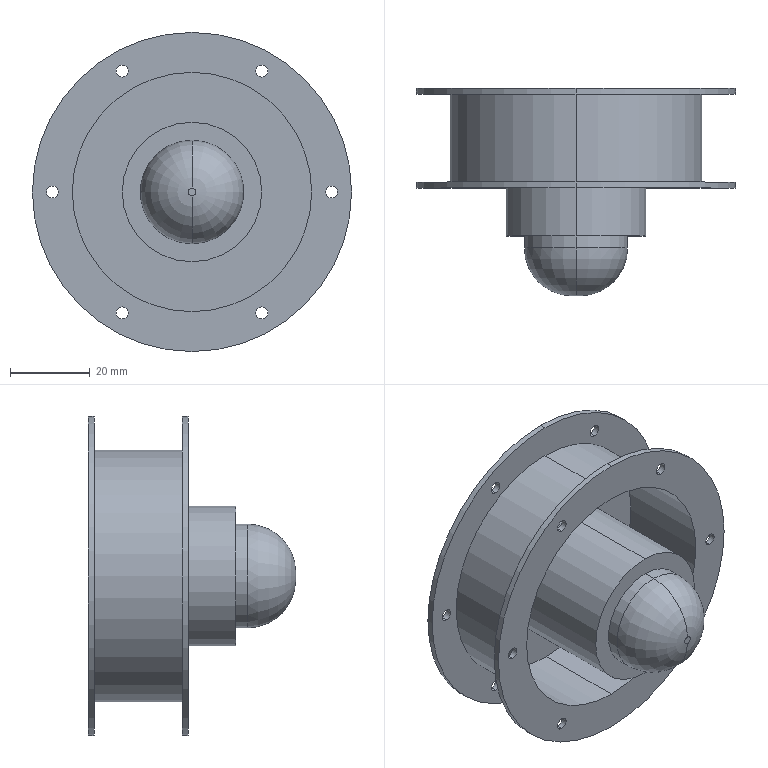Part | SolidWorks | features ICE 5, Fillet 1, Revolution 1 | 1 solid | 48 faces | box 80 x 52 x 80 mm | volume 58059 mm3 | cylinder 38 | plane 8 | torus 2 | commonest cylinder face diameters 3 x24 80 x4 6.964 x2 26 x2 35 x2 60 x2
STEP:
#1=CARTESIAN_POINT('',(0.,-15.,13.));
#2=VERTEX_POINT('',#1);
#3=CARTESIAN_POINT('',(0.,-15.,-13.));
#4=VERTEX_POINT('',#3);
#5=CARTESIAN_POINT('',(0.,-15.,0.));
#6=DIRECTION('',(0.,1.,0.));
#7=DIRECTION('',(0.,0.,-1.));
#8=AXIS2_PLACEMENT_3D('',#5,#6,#7);
#9=CIRCLE('',#8,13.);
#10=EDGE_CURVE('',#2,#4,#9,.T.);
#11=ORIENTED_EDGE('',*,*,#10,.F.);
#12=CARTESIAN_POINT('',(0.,-27.,1.));
#13=VERTEX_POINT('',#12);
#14=CARTESIAN_POINT('',(0.,-15.,1.));
#15=DIRECTION('',(1.,0.,0.));
#16=DIRECTION('',(0.,0.,-1.));
#17=AXIS2_PLACEMENT_3D('',#14,#15,#16);
#18=CIRCLE('',#17,12.);
#19=EDGE_CURVE('',#2,#13,#18,.T.);
#20=ORIENTED_EDGE('',*,*,#19,.T.);
#21=CARTESIAN_POINT('',(0.,-27.,-1.));
#22=VERTEX_POINT('',#21);
#23=CARTESIAN_POINT('',(0.,-27.,0.));
#24=DIRECTION('',(0.,-1.,0.));
#25=DIRECTION('',(0.,0.,-1.));
#26=AXIS2_PLACEMENT_3D('',#23,#24,#25);
#27=CIRCLE('',#26,1.);
#28=EDGE_CURVE('',#22,#13,#27,.T.);
#29=ORIENTED_EDGE('',*,*,#28,.F.);
#30=CARTESIAN_POINT('',(0.,-15.,-1.));
#31=DIRECTION('',(-1.,0.,0.));
#32=DIRECTION('',(0.,0.,1.));
#33=AXIS2_PLACEMENT_3D('',#30,#31,#32);
#34=CIRCLE('',#33,12.);
#35=EDGE_CURVE('',#4,#22,#34,.T.);
#36=ORIENTED_EDGE('',*,*,#35,.F.);
#37=EDGE_LOOP('',(#11,#20,#29,#36));
#38=FACE_OUTER_BOUND('',#37,.T.);
#39=CARTESIAN_POINT('',(0.,-15.,0.));
#40=DIRECTION('',(0.,-1.,0.));
#41=DIRECTION('',(0.,0.,-1.));
#42=AXIS2_PLACEMENT_3D('',#39,#40,#41);
#43=TOROIDAL_SURFACE('',#42,1.,12.);
#44=ADVANCED_FACE('',(#38),#43,.T.);
#45=ORIENTED_EDGE('',*,*,#10,.T.);
#46=CARTESIAN_POINT('',(0.,-12.,-13.));
#47=VERTEX_POINT('',#46);
#48=CARTESIAN_POINT('',(0.,-27.,-13.));
#49=DIRECTION('',(0.,1.,0.));
#50=VECTOR('',#49,1000.);
#51=LINE('',#48,#50);
#52=EDGE_CURVE('',#4,#47,#51,.T.);
#53=ORIENTED_EDGE('',*,*,#52,.T.);
#54=CARTESIAN_POINT('',(0.,-12.,13.));
#55=VERTEX_POINT('',#54);
#56=CARTESIAN_POINT('',(0.,-12.,0.));
#57=DIRECTION('',(0.,-1.,0.));
#58=DIRECTION('',(0.,0.,-1.));
#59=AXIS2_PLACEMENT_3D('',#56,#57,#58);
#60=CIRCLE('',#59,13.);
#61=EDGE_CURVE('',#47,#55,#60,.T.);
#62=ORIENTED_EDGE('',*,*,#61,.T.);
#63=CARTESIAN_POINT('',(0.,-27.,13.));
#64=DIRECTION('',(0.,1.,0.));
#65=VECTOR('',#64,1000.);
#66=LINE('',#63,#65);
#67=EDGE_CURVE('',#2,#55,#66,.T.);
#68=ORIENTED_EDGE('',*,*,#67,.F.);
#69=EDGE_LOOP('',(#45,#53,#62,#68));
#70=FACE_OUTER_BOUND('',#69,.T.);
#71=CARTESIAN_POINT('',(0.,-27.,0.));
#72=DIRECTION('',(0.,1.,0.));
#73=DIRECTION('',(0.,0.,1.));
#74=AXIS2_PLACEMENT_3D('',#71,#72,#73);
#75=CYLINDRICAL_SURFACE('',#74,13.);
#76=ADVANCED_FACE('',(#70),#75,.T.);
#77=CARTESIAN_POINT('',(0.,-12.,-17.5));
#78=VERTEX_POINT('',#77);
#79=CARTESIAN_POINT('',(0.,-12.,17.5));
#80=VERTEX_POINT('',#79);
#81=CARTESIAN_POINT('',(0.,-12.,0.));
#82=DIRECTION('',(0.,-1.,0.));
#83=DIRECTION('',(0.,0.,-1.));
#84=AXIS2_PLACEMENT_3D('',#81,#82,#83);
#85=CIRCLE('',#84,17.5);
#86=EDGE_CURVE('',#78,#80,#85,.T.);
#87=ORIENTED_EDGE('',*,*,#86,.F.);
#88=CARTESIAN_POINT('',(0.,23.,-17.5));
#89=VERTEX_POINT('',#88);
#90=CARTESIAN_POINT('',(0.,-12.,-17.5));
#91=DIRECTION('',(0.,1.,0.));
#92=VECTOR('',#91,1000.);
#93=LINE('',#90,#92);
#94=EDGE_CURVE('',#78,#89,#93,.T.);
#95=ORIENTED_EDGE('',*,*,#94,.T.);
#96=CARTESIAN_POINT('',(0.,23.,17.5));
#97=VERTEX_POINT('',#96);
#98=CARTESIAN_POINT('',(0.,23.,0.));
#99=DIRECTION('',(0.,-1.,0.));
#100=DIRECTION('',(0.,0.,1.));
#101=AXIS2_PLACEMENT_3D('',#98,#99,#100);
#102=CIRCLE('',#101,17.5);
#103=EDGE_CURVE('',#89,#97,#102,.T.);
#104=ORIENTED_EDGE('',*,*,#103,.T.);
#105=CARTESIAN_POINT('',(0.,-12.,17.5));
#106=DIRECTION('',(0.,1.,0.));
#107=VECTOR('',#106,1000.);
#108=LINE('',#105,#107);
#109=EDGE_CURVE('',#80,#97,#108,.T.);
#110=ORIENTED_EDGE('',*,*,#109,.F.);
#111=EDGE_LOOP('',(#87,#95,#104,#110));
#112=FACE_OUTER_BOUND('',#111,.T.);
#113=CARTESIAN_POINT('',(0.,-12.,0.));
#114=DIRECTION('',(0.,1.,0.));
#115=DIRECTION('',(0.,0.,1.));
#116=AXIS2_PLACEMENT_3D('',#113,#114,#115);
#117=CYLINDRICAL_SURFACE('',#116,17.5);
#118=ADVANCED_FACE('',(#112),#117,.T.);
#119=CARTESIAN_POINT('',(0.,25.,3.482));
#120=VERTEX_POINT('',#119);
#121=CARTESIAN_POINT('',(0.,25.,-3.482));
#122=VERTEX_POINT('',#121);
#123=CARTESIAN_POINT('',(0.,25.,0.));
#124=DIRECTION('',(0.,-1.,0.));
#125=DIRECTION('',(0.,0.,-1.));
#126=AXIS2_PLACEMENT_3D('',#123,#124,#125);
#127=CIRCLE('',#126,3.482);
#128=EDGE_CURVE('',#120,#122,#127,.T.);
#129=ORIENTED_EDGE('',*,*,#128,.F.);
#130=CARTESIAN_POINT('',(0.,23.,3.482));
#131=VERTEX_POINT('',#130);
#132=CARTESIAN_POINT('',(0.,25.,3.482));
#133=DIRECTION('',(0.,-1.,0.));
#134=VECTOR('',#133,1000.);
#135=LINE('',#132,#134);
#136=EDGE_CURVE('',#120,#131,#135,.T.);
#137=ORIENTED_EDGE('',*,*,#136,.T.);
#138=CARTESIAN_POINT('',(0.,23.,-3.482));
#139=VERTEX_POINT('',#138);
#140=CARTESIAN_POINT('',(0.,23.,0.));
#141=DIRECTION('',(0.,1.,0.));
#142=DIRECTION('',(0.,0.,-1.));
#143=AXIS2_PLACEMENT_3D('',#140,#141,#142);
#144=CIRCLE('',#143,3.482);
#145=EDGE_CURVE('',#139,#131,#144,.T.);
#146=ORIENTED_EDGE('',*,*,#145,.F.);
#147=CARTESIAN_POINT('',(0.,25.,-3.482));
#148=DIRECTION('',(0.,-1.,0.));
#149=VECTOR('',#148,1000.);
#150=LINE('',#147,#149);
#151=EDGE_CURVE('',#122,#139,#150,.T.);
#152=ORIENTED_EDGE('',*,*,#151,.F.);
#153=EDGE_LOOP('',(#129,#137,#146,#152));
#154=FACE_OUTER_BOUND('',#153,.T.);
#155=CARTESIAN_POINT('',(0.,25.,0.));
#156=DIRECTION('',(0.,-1.,0.));
#157=DIRECTION('',(0.,0.,-1.));
#158=AXIS2_PLACEMENT_3D('',#155,#156,#157);
#159=CYLINDRICAL_SURFACE('',#158,3.482);
#160=ADVANCED_FACE('',(#154),#159,.F.);
#161=CARTESIAN_POINT('',(-17.5,23.5,-31.811));
#162=VERTEX_POINT('',#161);
#163=CARTESIAN_POINT('',(-17.5,23.5,-28.811));
#164=VERTEX_POINT('',#163);
#165=CARTESIAN_POINT('',(-17.5,23.5,-30.311));
#166=DIRECTION('',(0.,1.,0.));
#167=DIRECTION('',(0.,0.,1.));
#168=AXIS2_PLACEMENT_3D('',#165,#166,#167);
#169=CIRCLE('',#168,1.5);
#170=EDGE_CURVE('',#162,#164,#169,.T.);
#171=ORIENTED_EDGE('',*,*,#170,.F.);
#172=CARTESIAN_POINT('',(-17.5,25.,-31.811));
#173=VERTEX_POINT('',#172);
#174=CARTESIAN_POINT('',(-17.5,0.,-31.811));
#175=DIRECTION('',(0.,1.,0.));
#176=VECTOR('',#175,1000.);
#177=LINE('',#174,#176);
#178=EDGE_CURVE('',#162,#173,#177,.T.);
#179=ORIENTED_EDGE('',*,*,#178,.T.);
#180=CARTESIAN_POINT('',(-17.5,25.,-28.811));
#181=VERTEX_POINT('',#180);
#182=CARTESIAN_POINT('',(-17.5,25.,-30.311));
#183=DIRECTION('',(0.,1.,0.));
#184=DIRECTION('',(0.,0.,1.));
#185=AXIS2_PLACEMENT_3D('',#182,#183,#184);
#186=CIRCLE('',#185,1.5);
#187=EDGE_CURVE('',#173,#181,#186,.T.);
#188=ORIENTED_EDGE('',*,*,#187,.T.);
#189=CARTESIAN_POINT('',(-17.5,0.,-28.811));
#190=DIRECTION('',(0.,1.,0.));
#191=VECTOR('',#190,1000.);
#192=LINE('',#189,#191);
#193=EDGE_CURVE('',#164,#181,#192,.T.);
#194=ORIENTED_EDGE('',*,*,#193,.F.);
#195=EDGE_LOOP('',(#171,#179,#188,#194));
#196=FACE_OUTER_BOUND('',#195,.T.);
#197=CARTESIAN_POINT('',(-17.5,0.,-30.311));
#198=DIRECTION('',(0.,1.,0.));
#199=DIRECTION('',(0.,0.,1.));
#200=AXIS2_PLACEMENT_3D('',#197,#198,#199);
#201=CYLINDRICAL_SURFACE('',#200,1.5);
#202=ADVANCED_FACE('',(#196),#201,.F.);
#203=CARTESIAN_POINT('',(17.5,23.5,-31.811));
#204=VERTEX_POINT('',#203);
#205=CARTESIAN_POINT('',(17.5,23.5,-28.811));
#206=VERTEX_POINT('',#205);
#207=CARTESIAN_POINT('',(17.5,23.5,-30.311));
#208=DIRECTION('',(0.,1.,0.));
#209=DIRECTION('',(0.,0.,1.));
#210=AXIS2_PLACEMENT_3D('',#207,#208,#209);
#211=CIRCLE('',#210,1.5);
#212=EDGE_CURVE('',#204,#206,#211,.T.);
#213=ORIENTED_EDGE('',*,*,#212,.F.);
#214=CARTESIAN_POINT('',(17.5,25.,-31.811));
#215=VERTEX_POINT('',#214);
#216=CARTESIAN_POINT('',(17.5,0.,-31.811));
#217=DIRECTION('',(0.,1.,0.));
#218=VECTOR('',#217,1000.);
#219=LINE('',#216,#218);
#220=EDGE_CURVE('',#204,#215,#219,.T.);
#221=ORIENTED_EDGE('',*,*,#220,.T.);
#222=CARTESIAN_POINT('',(17.5,25.,-28.811));
#223=VERTEX_POINT('',#222);
#224=CARTESIAN_POINT('',(17.5,25.,-30.311));
#225=DIRECTION('',(0.,1.,0.));
#226=DIRECTION('',(0.,0.,1.));
#227=AXIS2_PLACEMENT_3D('',#224,#225,#226);
#228=CIRCLE('',#227,1.5);
#229=EDGE_CURVE('',#215,#223,#228,.T.);
#230=ORIENTED_EDGE('',*,*,#229,.T.);
#231=CARTESIAN_POINT('',(17.5,0.,-28.811));
#232=DIRECTION('',(0.,1.,0.));
#233=VECTOR('',#232,1000.);
#234=LINE('',#231,#233);
#235=EDGE_CURVE('',#206,#223,#234,.T.);
#236=ORIENTED_EDGE('',*,*,#235,.F.);
#237=EDGE_LOOP('',(#213,#221,#230,#236));
#238=FACE_OUTER_BOUND('',#237,.T.);
#239=CARTESIAN_POINT('',(17.5,0.,-30.311));
#240=DIRECTION('',(0.,1.,0.));
#241=DIRECTION('',(0.,0.,1.));
#242=AXIS2_PLACEMENT_3D('',#239,#240,#241);
#243=CYLINDRICAL_SURFACE('',#242,1.5);
#244=ADVANCED_FACE('',(#238),#243,.F.);
#245=CARTESIAN_POINT('',(35.,23.5,-1.5));
#246=VERTEX_POINT('',#245);
#247=CARTESIAN_POINT('',(35.,23.5,1.5));
#248=VERTEX_POINT('',#247);
#249=CARTESIAN_POINT('',(35.,23.5,0.));
#250=DIRECTION('',(0.,1.,0.));
#251=DIRECTION('',(0.,0.,1.));
#252=AXIS2_PLACEMENT_3D('',#249,#250,#251);
#253=CIRCLE('',#252,1.5);
#254=EDGE_CURVE('',#246,#248,#253,.T.);
#255=ORIENTED_EDGE('',*,*,#254,.F.);
#256=CARTESIAN_POINT('',(35.,25.,-1.5));
#257=VERTEX_POINT('',#256);
#258=CARTESIAN_POINT('',(35.,0.,-1.5));
#259=DIRECTION('',(0.,1.,0.));
#260=VECTOR('',#259,1000.);
#261=LINE('',#258,#260);
#262=EDGE_CURVE('',#246,#257,#261,.T.);
#263=ORIENTED_EDGE('',*,*,#262,.T.);
#264=CARTESIAN_POINT('',(35.,25.,1.5));
#265=VERTEX_POINT('',#264);
#266=CARTESIAN_POINT('',(35.,25.,0.));
#267=DIRECTION('',(0.,1.,0.));
#268=DIRECTION('',(0.,0.,1.));
#269=AXIS2_PLACEMENT_3D('',#266,#267,#268);
#270=CIRCLE('',#269,1.5);
#271=EDGE_CURVE('',#257,#265,#270,.T.);
#272=ORIENTED_EDGE('',*,*,#271,.T.);
#273=CARTESIAN_POINT('',(35.,0.,1.5));
#274=DIRECTION('',(0.,1.,0.));
#275=VECTOR('',#274,1000.);
#276=LINE('',#273,#275);
#277=EDGE_CURVE('',#248,#265,#276,.T.);
#278=ORIENTED_EDGE('',*,*,#277,.F.);
#279=EDGE_LOOP('',(#255,#263,#272,#278));
#280=FACE_OUTER_BOUND('',#279,.T.);
#281=CARTESIAN_POINT('',(35.,0.,0.));
#282=DIRECTION('',(0.,1.,0.));
#283=DIRECTION('',(0.,0.,1.));
#284=AXIS2_PLACEMENT_3D('',#281,#282,#283);
#285=CYLINDRICAL_SURFACE('',#284,1.5);
#286=ADVANCED_FACE('',(#280),#285,.F.);
#287=CARTESIAN_POINT('',(17.5,23.5,28.811));
#288=VERTEX_POINT('',#287);
#289=CARTESIAN_POINT('',(17.5,23.5,31.811));
#290=VERTEX_POINT('',#289);
#291=CARTESIAN_POINT('',(17.5,23.5,30.311));
#292=DIRECTION('',(0.,1.,0.));
#293=DIRECTION('',(0.,0.,1.));
#294=AXIS2_PLACEMENT_3D('',#291,#292,#293);
#295=CIRCLE('',#294,1.5);
#296=EDGE_CURVE('',#288,#290,#295,.T.);
#297=ORIENTED_EDGE('',*,*,#296,.F.);
#298=CARTESIAN_POINT('',(17.5,25.,28.811));
#299=VERTEX_POINT('',#298);
#300=CARTESIAN_POINT('',(17.5,0.,28.811));
#301=DIRECTION('',(0.,1.,0.));
#302=VECTOR('',#301,1000.);
#303=LINE('',#300,#302);
#304=EDGE_CURVE('',#288,#299,#303,.T.);
#305=ORIENTED_EDGE('',*,*,#304,.T.);
#306=CARTESIAN_POINT('',(17.5,25.,31.811));
#307=VERTEX_POINT('',#306);
#308=CARTESIAN_POINT('',(17.5,25.,30.311));
#309=DIRECTION('',(0.,1.,0.));
#310=DIRECTION('',(0.,0.,1.));
#311=AXIS2_PLACEMENT_3D('',#308,#309,#310);
#312=CIRCLE('',#311,1.5);
#313=EDGE_CURVE('',#299,#307,#312,.T.);
#314=ORIENTED_EDGE('',*,*,#313,.T.);
#315=CARTESIAN_POINT('',(17.5,0.,31.811));
#316=DIRECTION('',(0.,1.,0.));
#317=VECTOR('',#316,1000.);
#318=LINE('',#315,#317);
#319=EDGE_CURVE('',#290,#307,#318,.T.);
#320=ORIENTED_EDGE('',*,*,#319,.F.);
#321=EDGE_LOOP('',(#297,#305,#314,#320));
#322=FACE_OUTER_BOUND('',#321,.T.);
#323=CARTESIAN_POINT('',(17.5,0.,30.311));
#324=DIRECTION('',(0.,1.,0.));
#325=DIRECTION('',(0.,0.,1.));
#326=AXIS2_PLACEMENT_3D('',#323,#324,#325);
#327=CYLINDRICAL_SURFACE('',#326,1.5);
#328=ADVANCED_FACE('',(#322),#327,.F.);
#329=CARTESIAN_POINT('',(-17.5,23.5,28.811));
#330=VERTEX_POINT('',#329);
#331=CARTESIAN_POINT('',(-17.5,23.5,31.811));
#332=VERTEX_POINT('',#331);
#333=CARTESIAN_POINT('',(-17.5,23.5,30.311));
#334=DIRECTION('',(0.,1.,0.));
#335=DIRECTION('',(0.,0.,1.));
#336=AXIS2_PLACEMENT_3D('',#333,#334,#335);
#337=CIRCLE('',#336,1.5);
#338=EDGE_CURVE('',#330,#332,#337,.T.);
#339=ORIENTED_EDGE('',*,*,#338,.F.);
#340=CARTESIAN_POINT('',(-17.5,25.,28.811));
#341=VERTEX_POINT('',#340);
#342=CARTESIAN_POINT('',(-17.5,0.,28.811));
#343=DIRECTION('',(0.,1.,0.));
#344=VECTOR('',#343,1000.);
#345=LINE('',#342,#344);
#346=EDGE_CURVE('',#330,#341,#345,.T.);
#347=ORIENTED_EDGE('',*,*,#346,.T.);
#348=CARTESIAN_POINT('',(-17.5,25.,31.811));
#349=VERTEX_POINT('',#348);
#350=CARTESIAN_POINT('',(-17.5,25.,30.311));
#351=DIRECTION('',(0.,1.,0.));
#352=DIRECTION('',(0.,0.,1.));
#353=AXIS2_PLACEMENT_3D('',#350,#351,#352);
#354=CIRCLE('',#353,1.5);
#355=EDGE_CURVE('',#341,#349,#354,.T.);
#356=ORIENTED_EDGE('',*,*,#355,.T.);
#357=CARTESIAN_POINT('',(-17.5,0.,31.811));
#358=DIRECTION('',(0.,1.,0.));
#359=VECTOR('',#358,1000.);
#360=LINE('',#357,#359);
#361=EDGE_CURVE('',#332,#349,#360,.T.);
#362=ORIENTED_EDGE('',*,*,#361,.F.);
#363=EDGE_LOOP('',(#339,#347,#356,#362));
#364=FACE_OUTER_BOUND('',#363,.T.);
#365=CARTESIAN_POINT('',(-17.5,0.,30.311));
#366=DIRECTION('',(0.,1.,0.));
#367=DIRECTION('',(0.,0.,1.));
#368=AXIS2_PLACEMENT_3D('',#365,#366,#367);
#369=CYLINDRICAL_SURFACE('',#368,1.5);
#370=ADVANCED_FACE('',(#364),#369,.F.);
#371=CARTESIAN_POINT('',(-17.5,0.,-31.811));
#372=VERTEX_POINT('',#371);
#373=CARTESIAN_POINT('',(-17.5,0.,-28.811));
#374=VERTEX_POINT('',#373);
#375=CARTESIAN_POINT('',(-17.5,0.,-30.311));
#376=DIRECTION('',(0.,1.,0.));
#377=DIRECTION('',(0.,0.,1.));
#378=AXIS2_PLACEMENT_3D('',#375,#376,#377);
#379=CIRCLE('',#378,1.5);
#380=EDGE_CURVE('',#372,#374,#379,.T.);
#381=ORIENTED_EDGE('',*,*,#380,.F.);
#382=CARTESIAN_POINT('',(-17.5,1.5,-31.811));
#383=VERTEX_POINT('',#382);
#384=CARTESIAN_POINT('',(-17.5,0.,-31.811));
#385=DIRECTION('',(0.,1.,0.));
#386=VECTOR('',#385,1000.);
#387=LINE('',#384,#386);
#388=EDGE_CURVE('',#372,#383,#387,.T.);
#389=ORIENTED_EDGE('',*,*,#388,.T.);
#390=CARTESIAN_POINT('',(-17.5,1.5,-28.811));
#391=VERTEX_POINT('',#390);
#392=CARTESIAN_POINT('',(-17.5,1.5,-30.311));
#393=DIRECTION('',(0.,-1.,0.));
#394=DIRECTION('',(0.,0.,-1.));
#395=AXIS2_PLACEMENT_3D('',#392,#393,#394);
#396=CIRCLE('',#395,1.5);
#397=EDGE_CURVE('',#391,#383,#396,.T.);
#398=ORIENTED_EDGE('',*,*,#397,.F.);
#399=CARTESIAN_POINT('',(-17.5,0.,-28.811));
#400=DIRECTION('',(0.,1.,0.));
#401=VECTOR('',#400,1000.);
#402=LINE('',#399,#401);
#403=EDGE_CURVE('',#374,#391,#402,.T.);
#404=ORIENTED_EDGE('',*,*,#403,.F.);
#405=EDGE_LOOP('',(#381,#389,#398,#404));
#406=FACE_OUTER_BOUND('',#405,.T.);
#407=CARTESIAN_POINT('',(-17.5,0.,-30.311));
#408=DIRECTION('',(0.,1.,0.));
#409=DIRECTION('',(0.,0.,1.));
#410=AXIS2_PLACEMENT_3D('',#407,#408,#409);
#411=CYLINDRICAL_SURFACE('',#410,1.5);
#412=ADVANCED_FACE('',(#406),#411,.F.);
#413=CARTESIAN_POINT('',(17.5,0.,-31.811));
#414=VERTEX_POINT('',#413);
#415=CARTESIAN_POINT('',(17.5,0.,-28.811));
#416=VERTEX_POINT('',#415);
#417=CARTESIAN_POINT('',(17.5,0.,-30.311));
#418=DIRECTION('',(0.,1.,0.));
#419=DIRECTION('',(0.,0.,1.));
#420=AXIS2_PLACEMENT_3D('',#417,#418,#419);
#421=CIRCLE('',#420,1.5);
#422=EDGE_CURVE('',#414,#416,#421,.T.);
#423=ORIENTED_EDGE('',*,*,#422,.F.);
#424=CARTESIAN_POINT('',(17.5,1.5,-31.811));
#425=VERTEX_POINT('',#424);
#426=CARTESIAN_POINT('',(17.5,0.,-31.811));
#427=DIRECTION('',(0.,1.,0.));
#428=VECTOR('',#427,1000.);
#429=LINE('',#426,#428);
#430=EDGE_CURVE('',#414,#425,#429,.T.);
#431=ORIENTED_EDGE('',*,*,#430,.T.);
#432=CARTESIAN_POINT('',(17.5,1.5,-28.811));
#433=VERTEX_POINT('',#432);
#434=CARTESIAN_POINT('',(17.5,1.5,-30.311));
#435=DIRECTION('',(0.,-1.,0.));
#436=DIRECTION('',(0.,0.,-1.));
#437=AXIS2_PLACEMENT_3D('',#434,#435,#436);
#438=CIRCLE('',#437,1.5);
#439=EDGE_CURVE('',#433,#425,#438,.T.);
#440=ORIENTED_EDGE('',*,*,#439,.F.);
#441=CARTESIAN_POINT('',(17.5,0.,-28.811));
#442=DIRECTION('',(0.,1.,0.));
#443=VECTOR('',#442,1000.);
#444=LINE('',#441,#443);
#445=EDGE_CURVE('',#416,#433,#444,.T.);
#446=ORIENTED_EDGE('',*,*,#445,.F.);
#447=EDGE_LOOP('',(#423,#431,#440,#446));
#448=FACE_OUTER_BOUND('',#447,.T.);
#449=CARTESIAN_POINT('',(17.5,0.,-30.311));
#450=DIRECTION('',(0.,1.,0.));
#451=DIRECTION('',(0.,0.,1.));
#452=AXIS2_PLACEMENT_3D('',#449,#450,#451);
#453=CYLINDRICAL_SURFACE('',#452,1.5);
#454=ADVANCED_FACE('',(#448),#453,.F.);
#455=CARTESIAN_POINT('',(35.,0.,-1.5));
#456=VERTEX_POINT('',#455);
#457=CARTESIAN_POINT('',(35.,0.,1.5));
#458=VERTEX_POINT('',#457);
#459=CARTESIAN_POINT('',(35.,0.,0.));
#460=DIRECTION('',(0.,1.,0.));
#461=DIRECTION('',(0.,0.,1.));
#462=AXIS2_PLACEMENT_3D('',#459,#460,#461);
#463=CIRCLE('',#462,1.5);
#464=EDGE_CURVE('',#456,#458,#463,.T.);
#465=ORIENTED_EDGE('',*,*,#464,.F.);
#466=CARTESIAN_POINT('',(35.,1.5,-1.5));
#467=VERTEX_POINT('',#466);
#468=CARTESIAN_POINT('',(35.,0.,-1.5));
#469=DIRECTION('',(0.,1.,0.));
#470=VECTOR('',#469,1000.);
#471=LINE('',#468,#470);
#472=EDGE_CURVE('',#456,#467,#471,.T.);
#473=ORIENTED_EDGE('',*,*,#472,.T.);
#474=CARTESIAN_POINT('',(35.,1.5,1.5));
#475=VERTEX_POINT('',#474);
#476=CARTESIAN_POINT('',(35.,1.5,0.));
#477=DIRECTION('',(0.,-1.,0.));
#478=DIRECTION('',(0.,0.,-1.));
#479=AXIS2_PLACEMENT_3D('',#476,#477,#478);
#480=CIRCLE('',#479,1.5);
#481=EDGE_CURVE('',#475,#467,#480,.T.);
#482=ORIENTED_EDGE('',*,*,#481,.F.);
#483=CARTESIAN_POINT('',(35.,0.,1.5));
#484=DIRECTION('',(0.,1.,0.));
#485=VECTOR('',#484,1000.);
#486=LINE('',#483,#485);
#487=EDGE_CURVE('',#458,#475,#486,.T.);
#488=ORIENTED_EDGE('',*,*,#487,.F.);
#489=EDGE_LOOP('',(#465,#473,#482,#488));
#490=FACE_OUTER_BOUND('',#489,.T.);
#491=CARTESIAN_POINT('',(35.,0.,0.));
#492=DIRECTION('',(0.,1.,0.));
#493=DIRECTION('',(0.,0.,1.));
#494=AXIS2_PLACEMENT_3D('',#491,#492,#493);
#495=CYLINDRICAL_SURFACE('',#494,1.5);
#496=ADVANCED_FACE('',(#490),#495,.F.);
#497=CARTESIAN_POINT('',(17.5,0.,28.811));
#498=VERTEX_POINT('',#497);
#499=CARTESIAN_POINT('',(17.5,0.,31.811));
#500=VERTEX_POINT('',#499);
#501=CARTESIAN_POINT('',(17.5,0.,30.311));
#502=DIRECTION('',(0.,1.,0.));
#503=DIRECTION('',(0.,0.,1.));
#504=AXIS2_PLACEMENT_3D('',#501,#502,#503);
#505=CIRCLE('',#504,1.5);
#506=EDGE_CURVE('',#498,#500,#505,.T.);
#507=ORIENTED_EDGE('',*,*,#506,.F.);
#508=CARTESIAN_POINT('',(17.5,1.5,28.811));
#509=VERTEX_POINT('',#508);
#510=CARTESIAN_POINT('',(17.5,0.,28.811));
#511=DIRECTION('',(0.,1.,0.));
#512=VECTOR('',#511,1000.);
#513=LINE('',#510,#512);
#514=EDGE_CURVE('',#498,#509,#513,.T.);
#515=ORIENTED_EDGE('',*,*,#514,.T.);
#516=CARTESIAN_POINT('',(17.5,1.5,31.811));
#517=VERTEX_POINT('',#516);
#518=CARTESIAN_POINT('',(17.5,1.5,30.311));
#519=DIRECTION('',(0.,-1.,0.));
#520=DIRECTION('',(0.,0.,-1.));
#521=AXIS2_PLACEMENT_3D('',#518,#519,#520);
#522=CIRCLE('',#521,1.5);
#523=EDGE_CURVE('',#517,#509,#522,.T.);
#524=ORIENTED_EDGE('',*,*,#523,.F.);
#525=CARTESIAN_POINT('',(17.5,0.,31.811));
#526=DIRECTION('',(0.,1.,0.));
#527=VECTOR('',#526,1000.);
#528=LINE('',#525,#527);
#529=EDGE_CURVE('',#500,#517,#528,.T.);
#530=ORIENTED_EDGE('',*,*,#529,.F.);
#531=EDGE_LOOP('',(#507,#515,#524,#530));
#532=FACE_OUTER_BOUND('',#531,.T.);
#533=CARTESIAN_POINT('',(17.5,0.,30.311));
#534=DIRECTION('',(0.,1.,0.));
#535=DIRECTION('',(0.,0.,1.));
#536=AXIS2_PLACEMENT_3D('',#533,#534,#535);
#537=CYLINDRICAL_SURFACE('',#536,1.5);
#538=ADVANCED_FACE('',(#532),#537,.F.);
#539=CARTESIAN_POINT('',(-17.5,0.,28.811));
#540=VERTEX_POINT('',#539);
#541=CARTESIAN_POINT('',(-17.5,0.,31.811));
#542=VERTEX_POINT('',#541);
#543=CARTESIAN_POINT('',(-17.5,0.,30.311));
#544=DIRECTION('',(0.,1.,0.));
#545=DIRECTION('',(0.,0.,1.));
#546=AXIS2_PLACEMENT_3D('',#543,#544,#545);
#547=CIRCLE('',#546,1.5);
#548=EDGE_CURVE('',#540,#542,#547,.T.);
#549=ORIENTED_EDGE('',*,*,#548,.F.);
#550=CARTESIAN_POINT('',(-17.5,1.5,28.811));
#551=VERTEX_POINT('',#550);
#552=CARTESIAN_POINT('',(-17.5,0.,28.811));
#553=DIRECTION('',(0.,1.,0.));
#554=VECTOR('',#553,1000.);
#555=LINE('',#552,#554);
#556=EDGE_CURVE('',#540,#551,#555,.T.);
#557=ORIENTED_EDGE('',*,*,#556,.T.);
#558=CARTESIAN_POINT('',(-17.5,1.5,31.811));
#559=VERTEX_POINT('',#558);
#560=CARTESIAN_POINT('',(-17.5,1.5,30.311));
#561=DIRECTION('',(0.,-1.,0.));
#562=DIRECTION('',(0.,0.,-1.));
#563=AXIS2_PLACEMENT_3D('',#560,#561,#562);
#564=CIRCLE('',#563,1.5);
#565=EDGE_CURVE('',#559,#551,#564,.T.);
#566=ORIENTED_EDGE('',*,*,#565,.F.);
#567=CARTESIAN_POINT('',(-17.5,0.,31.811));
#568=DIRECTION('',(0.,1.,0.));
#569=VECTOR('',#568,1000.);
#570=LINE('',#567,#569);
#571=EDGE_CURVE('',#542,#559,#570,.T.);
#572=ORIENTED_EDGE('',*,*,#571,.F.);
#573=EDGE_LOOP('',(#549,#557,#566,#572));
#574=FACE_OUTER_BOUND('',#573,.T.);
#575=CARTESIAN_POINT('',(-17.5,0.,30.311));
#576=DIRECTION('',(0.,1.,0.));
#577=DIRECTION('',(0.,0.,1.));
#578=AXIS2_PLACEMENT_3D('',#575,#576,#577);
#579=CYLINDRICAL_SURFACE('',#578,1.5);
#580=ADVANCED_FACE('',(#574),#579,.F.);
#581=CARTESIAN_POINT('',(-35.,23.5,-1.5));
#582=VERTEX_POINT('',#581);
#583=CARTESIAN_POINT('',(-35.,23.5,1.5));
#584=VERTEX_POINT('',#583);
#585=CARTESIAN_POINT('',(-35.,23.5,0.));
#586=DIRECTION('',(0.,1.,0.));
#587=DIRECTION('',(0.,0.,1.));
#588=AXIS2_PLACEMENT_3D('',#585,#586,#587);
#589=CIRCLE('',#588,1.5);
#590=EDGE_CURVE('',#582,#584,#589,.T.);
#591=ORIENTED_EDGE('',*,*,#590,.F.);
#592=CARTESIAN_POINT('',(-35.,25.,-1.5));
#593=VERTEX_POINT('',#592);
#594=CARTESIAN_POINT('',(-35.,0.,-1.5));
#595=DIRECTION('',(0.,1.,0.));
#596=VECTOR('',#595,1000.);
#597=LINE('',#594,#596);
#598=EDGE_CURVE('',#582,#593,#597,.T.);
#599=ORIENTED_EDGE('',*,*,#598,.T.);
#600=CARTESIAN_POINT('',(-35.,25.,1.5));
#601=VERTEX_POINT('',#600);
#602=CARTESIAN_POINT('',(-35.,25.,0.));
#603=DIRECTION('',(0.,1.,0.));
#604=DIRECTION('',(0.,0.,1.));
#605=AXIS2_PLACEMENT_3D('',#602,#603,#604);
#606=CIRCLE('',#605,1.5);
#607=EDGE_CURVE('',#593,#601,#606,.T.);
#608=ORIENTED_EDGE('',*,*,#607,.T.);
#609=CARTESIAN_POINT('',(-35.,0.,1.5));
#610=DIRECTION('',(0.,1.,0.));
#611=VECTOR('',#610,1000.);
#612=LINE('',#609,#611);
#613=EDGE_CURVE('',#584,#601,#612,.T.);
#614=ORIENTED_EDGE('',*,*,#613,.F.);
#615=EDGE_LOOP('',(#591,#599,#608,#614));
#616=FACE_OUTER_BOUND('',#615,.T.);
#617=CARTESIAN_POINT('',(-35.,0.,0.));
#618=DIRECTION('',(0.,1.,0.));
#619=DIRECTION('',(0.,0.,1.));
#620=AXIS2_PLACEMENT_3D('',#617,#618,#619);
#621=CYLINDRICAL_SURFACE('',#620,1.5);
#622=ADVANCED_FACE('',(#616),#621,.F.);
#623=CARTESIAN_POINT('',(-35.,0.,-1.5));
#624=VERTEX_POINT('',#623);
#625=CARTESIAN_POINT('',(-35.,0.,1.5));
#626=VERTEX_POINT('',#625);
#627=CARTESIAN_POINT('',(-35.,0.,0.));
#628=DIRECTION('',(0.,1.,0.));
#629=DIRECTION('',(0.,0.,1.));
#630=AXIS2_PLACEMENT_3D('',#627,#628,#629);
#631=CIRCLE('',#630,1.5);
#632=EDGE_CURVE('',#624,#626,#631,.T.);
#633=ORIENTED_EDGE('',*,*,#632,.F.);
#634=CARTESIAN_POINT('',(-35.,1.5,-1.5));
#635=VERTEX_POINT('',#634);
#636=CARTESIAN_POINT('',(-35.,0.,-1.5));
#637=DIRECTION('',(0.,1.,0.));
#638=VECTOR('',#637,1000.);
#639=LINE('',#636,#638);
#640=EDGE_CURVE('',#624,#635,#639,.T.);
#641=ORIENTED_EDGE('',*,*,#640,.T.);
#642=CARTESIAN_POINT('',(-35.,1.5,1.5));
#643=VERTEX_POINT('',#642);
#644=CARTESIAN_POINT('',(-35.,1.5,0.));
#645=DIRECTION('',(0.,-1.,0.));
#646=DIRECTION('',(0.,0.,-1.));
#647=AXIS2_PLACEMENT_3D('',#644,#645,#646);
#648=CIRCLE('',#647,1.5);
#649=EDGE_CURVE('',#643,#635,#648,.T.);
#650=ORIENTED_EDGE('',*,*,#649,.F.);
#651=CARTESIAN_POINT('',(-35.,0.,1.5));
#652=DIRECTION('',(0.,1.,0.));
#653=VECTOR('',#652,1000.);
#654=LINE('',#651,#653);
#655=EDGE_CURVE('',#626,#643,#654,.T.);
#656=ORIENTED_EDGE('',*,*,#655,.F.);
#657=EDGE_LOOP('',(#633,#641,#650,#656));
#658=FACE_OUTER_BOUND('',#657,.T.);
#659=CARTESIAN_POINT('',(-35.,0.,0.));
#660=DIRECTION('',(0.,1.,0.));
#661=DIRECTION('',(0.,0.,1.));
#662=AXIS2_PLACEMENT_3D('',#659,#660,#661);
#663=CYLINDRICAL_SURFACE('',#662,1.5);
#664=ADVANCED_FACE('',(#658),#663,.F.);
#665=CARTESIAN_POINT('',(0.,23.5,-31.5));
#666=VERTEX_POINT('',#665);
#667=CARTESIAN_POINT('',(0.,23.5,31.5));
#668=VERTEX_POINT('',#667);
#669=CARTESIAN_POINT('',(0.,23.5,0.));
#670=DIRECTION('',(0.,-1.,0.));
#671=DIRECTION('',(0.,0.,-1.));
#672=AXIS2_PLACEMENT_3D('',#669,#670,#671);
#673=CIRCLE('',#672,31.5);
#674=EDGE_CURVE('',#666,#668,#673,.T.);
#675=ORIENTED_EDGE('',*,*,#674,.T.);
#676=CARTESIAN_POINT('',(0.,1.5,31.5));
#677=VERTEX_POINT('',#676);
#678=CARTESIAN_POINT('',(0.,0.,31.5));
#679=DIRECTION('',(0.,-1.,0.));
#680=VECTOR('',#679,1000.);
#681=LINE('',#678,#680);
#682=EDGE_CURVE('',#668,#677,#681,.T.);
#683=ORIENTED_EDGE('',*,*,#682,.T.);
#684=CARTESIAN_POINT('',(0.,1.5,-31.5));
#685=VERTEX_POINT('',#684);
#686=CARTESIAN_POINT('',(0.,1.5,0.));
#687=DIRECTION('',(0.,-1.,0.));
#688=DIRECTION('',(0.,0.,-1.));
#689=AXIS2_PLACEMENT_3D('',#686,#687,#688);
#690=CIRCLE('',#689,31.5);
#691=EDGE_CURVE('',#685,#677,#690,.T.);
#692=ORIENTED_EDGE('',*,*,#691,.F.);
#693=CARTESIAN_POINT('',(0.,0.,-31.5));
#694=DIRECTION('',(0.,-1.,0.));
#695=VECTOR('',#694,1000.);
#696=LINE('',#693,#695);
#697=EDGE_CURVE('',#666,#685,#696,.T.);
#698=ORIENTED_EDGE('',*,*,#697,.F.);
#699=EDGE_LOOP('',(#675,#683,#692,#698));
#700=FACE_OUTER_BOUND('',#699,.T.);
#701=CARTESIAN_POINT('',(0.,0.,0.));
#702=DIRECTION('',(0.,-1.,0.));
#703=DIRECTION('',(0.,0.,-1.));
#704=AXIS2_PLACEMENT_3D('',#701,#702,#703);
#705=CYLINDRICAL_SURFACE('',#704,31.5);
#706=ADVANCED_FACE('',(#700),#705,.T.);
#707=CARTESIAN_POINT('',(0.,25.,-40.));
#708=VERTEX_POINT('',#707);
#709=CARTESIAN_POINT('',(0.,25.,40.));
#710=VERTEX_POINT('',#709);
#711=CARTESIAN_POINT('',(0.,25.,0.));
#712=DIRECTION('',(0.,-1.,0.));
#713=DIRECTION('',(0.,0.,-1.));
#714=AXIS2_PLACEMENT_3D('',#711,#712,#713);
#715=CIRCLE('',#714,40.);
#716=EDGE_CURVE('',#708,#710,#715,.T.);
#717=ORIENTED_EDGE('',*,*,#716,.T.);
#718=CARTESIAN_POINT('',(0.,23.5,40.));
#719=VERTEX_POINT('',#718);
#720=CARTESIAN_POINT('',(0.,0.,40.));
#721=DIRECTION('',(0.,-1.,0.));
#722=VECTOR('',#721,1000.);
#723=LINE('',#720,#722);
#724=EDGE_CURVE('',#710,#719,#723,.T.);
#725=ORIENTED_EDGE('',*,*,#724,.T.);
#726=CARTESIAN_POINT('',(0.,23.5,-40.));
#727=VERTEX_POINT('',#726);
#728=CARTESIAN_POINT('',(0.,23.5,0.));
#729=DIRECTION('',(0.,-1.,0.));
#730=DIRECTION('',(0.,0.,-1.));
#731=AXIS2_PLACEMENT_3D('',#728,#729,#730);
#732=CIRCLE('',#731,40.);
#733=EDGE_CURVE('',#727,#719,#732,.T.);
#734=ORIENTED_EDGE('',*,*,#733,.F.);
#735=CARTESIAN_POINT('',(0.,0.,-40.));
#736=DIRECTION('',(0.,-1.,0.));
#737=VECTOR('',#736,1000.);
#738=LINE('',#735,#737);
#739=EDGE_CURVE('',#708,#727,#738,.T.);
#740=ORIENTED_EDGE('',*,*,#739,.F.);
#741=EDGE_LOOP('',(#717,#725,#734,#740));
#742=FACE_OUTER_BOUND('',#741,.T.);
#743=CARTESIAN_POINT('',(0.,0.,0.));
#744=DIRECTION('',(0.,-1.,0.));
#745=DIRECTION('',(0.,0.,-1.));
#746=AXIS2_PLACEMENT_3D('',#743,#744,#745);
#747=CYLINDRICAL_SURFACE('',#746,40.);
#748=ADVANCED_FACE('',(#742),#747,.T.);
#749=CARTESIAN_POINT('',(0.,1.5,-40.));
#750=VERTEX_POINT('',#749);
#751=CARTESIAN_POINT('',(0.,1.5,40.));
#752=VERTEX_POINT('',#751);
#753=CARTESIAN_POINT('',(0.,1.5,0.));
#754=DIRECTION('',(0.,-1.,0.));
#755=DIRECTION('',(0.,0.,-1.));
#756=AXIS2_PLACEMENT_3D('',#753,#754,#755);
#757=CIRCLE('',#756,40.);
#758=EDGE_CURVE('',#750,#752,#757,.T.);
#759=ORIENTED_EDGE('',*,*,#758,.T.);
#760=CARTESIAN_POINT('',(0.,0.,40.));
#761=VERTEX_POINT('',#760);
#762=CARTESIAN_POINT('',(0.,0.,40.));
#763=DIRECTION('',(0.,-1.,0.));
#764=VECTOR('',#763,1000.);
#765=LINE('',#762,#764);
#766=EDGE_CURVE('',#752,#761,#765,.T.);
#767=ORIENTED_EDGE('',*,*,#766,.T.);
#768=CARTESIAN_POINT('',(0.,0.,-40.));
#769=VERTEX_POINT('',#768);
#770=CARTESIAN_POINT('',(0.,0.,0.));
#771=DIRECTION('',(0.,-1.,0.));
#772=DIRECTION('',(0.,0.,-1.));
#773=AXIS2_PLACEMENT_3D('',#770,#771,#772);
#774=CIRCLE('',#773,40.);
#775=EDGE_CURVE('',#769,#761,#774,.T.);
#776=ORIENTED_EDGE('',*,*,#775,.F.);
#777=CARTESIAN_POINT('',(0.,0.,-40.));
#778=DIRECTION('',(0.,-1.,0.));
#779=VECTOR('',#778,1000.);
#780=LINE('',#777,#779);
#781=EDGE_CURVE('',#750,#769,#780,.T.);
#782=ORIENTED_EDGE('',*,*,#781,.F.);
#783=EDGE_LOOP('',(#759,#767,#776,#782));
#784=FACE_OUTER_BOUND('',#783,.T.);
#785=CARTESIAN_POINT('',(0.,0.,0.));
#786=DIRECTION('',(0.,-1.,0.));
#787=DIRECTION('',(0.,0.,-1.));
#788=AXIS2_PLACEMENT_3D('',#785,#786,#787);
#789=CYLINDRICAL_SURFACE('',#788,40.);
#790=ADVANCED_FACE('',(#784),#789,.T.);
#791=CARTESIAN_POINT('',(0.,23.,30.));
#792=VERTEX_POINT('',#791);
#793=CARTESIAN_POINT('',(0.,23.,-30.));
#794=VERTEX_POINT('',#793);
#795=CARTESIAN_POINT('',(0.,23.,0.));
#796=DIRECTION('',(0.,-1.,0.));
#797=DIRECTION('',(0.,0.,1.));
#798=AXIS2_PLACEMENT_3D('',#795,#796,#797);
#799=CIRCLE('',#798,30.);
#800=EDGE_CURVE('',#792,#794,#799,.T.);
#801=ORIENTED_EDGE('',*,*,#800,.F.);
#802=CARTESIAN_POINT('',(0.,0.,30.));
#803=VERTEX_POINT('',#802);
#804=CARTESIAN_POINT('',(0.,0.,30.));
#805=DIRECTION('',(0.,-1.,0.));
#806=VECTOR('',#805,1000.);
#807=LINE('',#804,#806);
#808=EDGE_CURVE('',#792,#803,#807,.T.);
#809=ORIENTED_EDGE('',*,*,#808,.T.);
#810=CARTESIAN_POINT('',(0.,0.,-30.));
#811=VERTEX_POINT('',#810);
#812=CARTESIAN_POINT('',(0.,0.,0.));
#813=DIRECTION('',(0.,-1.,0.));
#814=DIRECTION('',(0.,0.,-1.));
#815=AXIS2_PLACEMENT_3D('',#812,#813,#814);
#816=CIRCLE('',#815,30.);
#817=EDGE_CURVE('',#803,#811,#816,.T.);
#818=ORIENTED_EDGE('',*,*,#817,.T.);
#819=CARTESIAN_POINT('',(0.,0.,-30.));
#820=DIRECTION('',(0.,-1.,0.));
#821=VECTOR('',#820,1000.);
#822=LINE('',#819,#821);
#823=EDGE_CURVE('',#794,#811,#822,.T.);
#824=ORIENTED_EDGE('',*,*,#823,.F.);
#825=EDGE_LOOP('',(#801,#809,#818,#824));
#826=FACE_OUTER_BOUND('',#825,.T.);
#827=CARTESIAN_POINT('',(0.,0.,0.));
#828=DIRECTION('',(0.,-1.,0.));
#829=DIRECTION('',(0.,0.,-1.));
#830=AXIS2_PLACEMENT_3D('',#827,#828,#829);
#831=CYLINDRICAL_SURFACE('',#830,30.);
#832=ADVANCED_FACE('',(#826),#831,.F.);
#833=ORIENTED_EDGE('',*,*,#808,.F.);
#834=CARTESIAN_POINT('',(0.,23.,0.));
#835=DIRECTION('',(0.,-1.,0.));
#836=DIRECTION('',(0.,0.,1.));
#837=AXIS2_PLACEMENT_3D('',#834,#835,#836);
#838=CIRCLE('',#837,30.);
#839=EDGE_CURVE('',#794,#792,#838,.T.);
#840=ORIENTED_EDGE('',*,*,#839,.F.);
#841=ORIENTED_EDGE('',*,*,#823,.T.);
#842=CARTESIAN_POINT('',(0.,0.,0.));
#843=DIRECTION('',(0.,-1.,0.));
#844=DIRECTION('',(0.,0.,-1.));
#845=AXIS2_PLACEMENT_3D('',#842,#843,#844);
#846=CIRCLE('',#845,30.);
#847=EDGE_CURVE('',#811,#803,#846,.T.);
#848=ORIENTED_EDGE('',*,*,#847,.T.);
#849=EDGE_LOOP('',(#833,#840,#841,#848));
#850=FACE_OUTER_BOUND('',#849,.T.);
#851=CARTESIAN_POINT('',(0.,0.,0.));
#852=DIRECTION('',(0.,-1.,0.));
#853=DIRECTION('',(0.,0.,-1.));
#854=AXIS2_PLACEMENT_3D('',#851,#852,#853);
#855=CYLINDRICAL_SURFACE('',#854,30.);
#856=ADVANCED_FACE('',(#850),#855,.F.);
#857=ORIENTED_EDGE('',*,*,#766,.F.);
#858=CARTESIAN_POINT('',(0.,1.5,0.));
#859=DIRECTION('',(0.,-1.,0.));
#860=DIRECTION('',(0.,0.,-1.));
#861=AXIS2_PLACEMENT_3D('',#858,#859,#860);
#862=CIRCLE('',#861,40.);
#863=EDGE_CURVE('',#752,#750,#862,.T.);
#864=ORIENTED_EDGE('',*,*,#863,.T.);
#865=ORIENTED_EDGE('',*,*,#781,.T.);
#866=CARTESIAN_POINT('',(0.,0.,0.));
#867=DIRECTION('',(0.,-1.,0.));
#868=DIRECTION('',(0.,0.,-1.));
#869=AXIS2_PLACEMENT_3D('',#866,#867,#868);
#870=CIRCLE('',#869,40.);
#871=EDGE_CURVE('',#761,#769,#870,.T.);
#872=ORIENTED_EDGE('',*,*,#871,.F.);
#873=EDGE_LOOP('',(#857,#864,#865,#872));
#874=FACE_OUTER_BOUND('',#873,.T.);
#875=CARTESIAN_POINT('',(0.,0.,0.));
#876=DIRECTION('',(0.,-1.,0.));
#877=DIRECTION('',(0.,0.,-1.));
#878=AXIS2_PLACEMENT_3D('',#875,#876,#877);
#879=CYLINDRICAL_SURFACE('',#878,40.);
#880=ADVANCED_FACE('',(#874),#879,.T.);
#881=CARTESIAN_POINT('',(-17.5,0.,-30.311));
#882=DIRECTION('',(0.,1.,0.));
#883=DIRECTION('',(0.,0.,1.));
#884=AXIS2_PLACEMENT_3D('',#881,#882,#883);
#885=CIRCLE('',#884,1.5);
#886=EDGE_CURVE('',#374,#372,#885,.T.);
#887=ORIENTED_EDGE('',*,*,#886,.T.);
#888=ORIENTED_EDGE('',*,*,#380,.T.);
#889=EDGE_LOOP('',(#887,#888));
#890=FACE_BOUND('',#889,.T.);
#891=CARTESIAN_POINT('',(17.5,0.,-30.311));
#892=DIRECTION('',(0.,1.,0.));
#893=DIRECTION('',(0.,0.,1.));
#894=AXIS2_PLACEMENT_3D('',#891,#892,#893);
#895=CIRCLE('',#894,1.5);
#896=EDGE_CURVE('',#416,#414,#895,.T.);
#897=ORIENTED_EDGE('',*,*,#896,.T.);
#898=ORIENTED_EDGE('',*,*,#422,.T.);
#899=EDGE_LOOP('',(#897,#898));
#900=FACE_BOUND('',#899,.T.);
#901=CARTESIAN_POINT('',(35.,0.,0.));
#902=DIRECTION('',(0.,1.,0.));
#903=DIRECTION('',(0.,0.,1.));
#904=AXIS2_PLACEMENT_3D('',#901,#902,#903);
#905=CIRCLE('',#904,1.5);
#906=EDGE_CURVE('',#458,#456,#905,.T.);
#907=ORIENTED_EDGE('',*,*,#906,.T.);
#908=ORIENTED_EDGE('',*,*,#464,.T.);
#909=EDGE_LOOP('',(#907,#908));
#910=FACE_BOUND('',#909,.T.);
#911=CARTESIAN_POINT('',(17.5,0.,30.311));
#912=DIRECTION('',(0.,1.,0.));
#913=DIRECTION('',(0.,0.,1.));
#914=AXIS2_PLACEMENT_3D('',#911,#912,#913);
#915=CIRCLE('',#914,1.5);
#916=EDGE_CURVE('',#500,#498,#915,.T.);
#917=ORIENTED_EDGE('',*,*,#916,.T.);
#918=ORIENTED_EDGE('',*,*,#506,.T.);
#919=EDGE_LOOP('',(#917,#918));
#920=FACE_BOUND('',#919,.T.);
#921=CARTESIAN_POINT('',(-17.5,0.,30.311));
#922=DIRECTION('',(0.,1.,0.));
#923=DIRECTION('',(0.,0.,1.));
#924=AXIS2_PLACEMENT_3D('',#921,#922,#923);
#925=CIRCLE('',#924,1.5);
#926=EDGE_CURVE('',#542,#540,#925,.T.);
#927=ORIENTED_EDGE('',*,*,#926,.T.);
#928=ORIENTED_EDGE('',*,*,#548,.T.);
#929=EDGE_LOOP('',(#927,#928));
#930=FACE_BOUND('',#929,.T.);
#931=CARTESIAN_POINT('',(-35.,0.,0.));
#932=DIRECTION('',(0.,1.,0.));
#933=DIRECTION('',(0.,0.,1.));
#934=AXIS2_PLACEMENT_3D('',#931,#932,#933);
#935=CIRCLE('',#934,1.5);
#936=EDGE_CURVE('',#626,#624,#935,.T.);
#937=ORIENTED_EDGE('',*,*,#936,.T.);
#938=ORIENTED_EDGE('',*,*,#632,.T.);
#939=EDGE_LOOP('',(#937,#938));
#940=FACE_BOUND('',#939,.T.);
#941=ORIENTED_EDGE('',*,*,#847,.F.);
#942=ORIENTED_EDGE('',*,*,#817,.F.);
#943=EDGE_LOOP('',(#941,#942));
#944=FACE_BOUND('',#943,.T.);
#945=ORIENTED_EDGE('',*,*,#775,.T.);
#946=ORIENTED_EDGE('',*,*,#871,.T.);
#947=EDGE_LOOP('',(#945,#946));
#948=FACE_OUTER_BOUND('',#947,.T.);
#949=CARTESIAN_POINT('',(-40.,0.,0.));
#950=DIRECTION('',(0.,1.,0.));
#951=DIRECTION('',(0.,0.,1.));
#952=AXIS2_PLACEMENT_3D('',#949,#950,#951);
#953=PLANE('',#952);
#954=ADVANCED_FACE('',(#890,#900,#910,#920,#930,#940,#944,#948),#953,.F.);
#955=CARTESIAN_POINT('',(0.,25.,0.));
#956=DIRECTION('',(0.,-1.,0.));
#957=DIRECTION('',(0.,0.,-1.));
#958=AXIS2_PLACEMENT_3D('',#955,#956,#957);
#959=CIRCLE('',#958,3.482);
#960=EDGE_CURVE('',#122,#120,#959,.T.);
#961=ORIENTED_EDGE('',*,*,#960,.T.);
#962=ORIENTED_EDGE('',*,*,#128,.T.);
#963=EDGE_LOOP('',(#961,#962));
#964=FACE_BOUND('',#963,.T.);
#965=CARTESIAN_POINT('',(-17.5,25.,-30.311));
#966=DIRECTION('',(0.,1.,0.));
#967=DIRECTION('',(0.,0.,1.));
#968=AXIS2_PLACEMENT_3D('',#965,#966,#967);
#969=CIRCLE('',#968,1.5);
#970=EDGE_CURVE('',#181,#173,#969,.T.);
#971=ORIENTED_EDGE('',*,*,#970,.F.);
#972=ORIENTED_EDGE('',*,*,#187,.F.);
#973=EDGE_LOOP('',(#971,#972));
#974=FACE_BOUND('',#973,.T.);
#975=CARTESIAN_POINT('',(17.5,25.,-30.311));
#976=DIRECTION('',(0.,1.,0.));
#977=DIRECTION('',(0.,0.,1.));
#978=AXIS2_PLACEMENT_3D('',#975,#976,#977);
#979=CIRCLE('',#978,1.5);
#980=EDGE_CURVE('',#223,#215,#979,.T.);
#981=ORIENTED_EDGE('',*,*,#980,.F.);
#982=ORIENTED_EDGE('',*,*,#229,.F.);
#983=EDGE_LOOP('',(#981,#982));
#984=FACE_BOUND('',#983,.T.);
#985=CARTESIAN_POINT('',(35.,25.,0.));
#986=DIRECTION('',(0.,1.,0.));
#987=DIRECTION('',(0.,0.,1.));
#988=AXIS2_PLACEMENT_3D('',#985,#986,#987);
#989=CIRCLE('',#988,1.5);
#990=EDGE_CURVE('',#265,#257,#989,.T.);
#991=ORIENTED_EDGE('',*,*,#990,.F.);
#992=ORIENTED_EDGE('',*,*,#271,.F.);
#993=EDGE_LOOP('',(#991,#992));
#994=FACE_BOUND('',#993,.T.);
#995=CARTESIAN_POINT('',(17.5,25.,30.311));
#996=DIRECTION('',(0.,1.,0.));
#997=DIRECTION('',(0.,0.,1.));
#998=AXIS2_PLACEMENT_3D('',#995,#996,#997);
#999=CIRCLE('',#998,1.5);
#1000=EDGE_CURVE('',#307,#299,#999,.T.);
#1001=ORIENTED_EDGE('',*,*,#1000,.F.);
#1002=ORIENTED_EDGE('',*,*,#313,.F.);
#1003=EDGE_LOOP('',(#1001,#1002));
#1004=FACE_BOUND('',#1003,.T.);
#1005=CARTESIAN_POINT('',(-17.5,25.,30.311));
#1006=DIRECTION('',(0.,1.,0.));
#1007=DIRECTION('',(0.,0.,1.));
#1008=AXIS2_PLACEMENT_3D('',#1005,#1006,#1007);
#1009=CIRCLE('',#1008,1.5);
#1010=EDGE_CURVE('',#349,#341,#1009,.T.);
#1011=ORIENTED_EDGE('',*,*,#1010,.F.);
#1012=ORIENTED_EDGE('',*,*,#355,.F.);
#1013=EDGE_LOOP('',(#1011,#1012));
#1014=FACE_BOUND('',#1013,.T.);
#1015=CARTESIAN_POINT('',(-35.,25.,0.));
#1016=DIRECTION('',(0.,1.,0.));
#1017=DIRECTION('',(0.,0.,1.));
#1018=AXIS2_PLACEMENT_3D('',#1015,#1016,#1017);
#1019=CIRCLE('',#1018,1.5);
#1020=EDGE_CURVE('',#601,#593,#1019,.T.);
#1021=ORIENTED_EDGE('',*,*,#1020,.F.);
#1022=ORIENTED_EDGE('',*,*,#607,.F.);
#1023=EDGE_LOOP('',(#1021,#1022));
#1024=FACE_BOUND('',#1023,.T.);
#1025=ORIENTED_EDGE('',*,*,#716,.F.);
#1026=CARTESIAN_POINT('',(0.,25.,0.));
#1027=DIRECTION('',(0.,-1.,0.));
#1028=DIRECTION('',(0.,0.,-1.));
#1029=AXIS2_PLACEMENT_3D('',#1026,#1027,#1028);
#1030=CIRCLE('',#1029,40.);
#1031=EDGE_CURVE('',#710,#708,#1030,.T.);
#1032=ORIENTED_EDGE('',*,*,#1031,.F.);
#1033=EDGE_LOOP('',(#1025,#1032));
#1034=FACE_OUTER_BOUND('',#1033,.T.);
#1035=CARTESIAN_POINT('',(-40.,25.,0.));
#1036=DIRECTION('',(0.,-1.,0.));
#1037=DIRECTION('',(0.,0.,-1.));
#1038=AXIS2_PLACEMENT_3D('',#1035,#1036,#1037);
#1039=PLANE('',#1038);
#1040=ADVANCED_FACE('',(#964,#974,#984,#994,#1004,#1014,#1024,#1034),#1039,.F.);
#1041=ORIENTED_EDGE('',*,*,#724,.F.);
#1042=ORIENTED_EDGE('',*,*,#1031,.T.);
#1043=ORIENTED_EDGE('',*,*,#739,.T.);
#1044=CARTESIAN_POINT('',(0.,23.5,0.));
#1045=DIRECTION('',(0.,-1.,0.));
#1046=DIRECTION('',(0.,0.,-1.));
#1047=AXIS2_PLACEMENT_3D('',#1044,#1045,#1046);
#1048=CIRCLE('',#1047,40.);
#1049=EDGE_CURVE('',#719,#727,#1048,.T.);
#1050=ORIENTED_EDGE('',*,*,#1049,.F.);
#1051=EDGE_LOOP('',(#1041,#1042,#1043,#1050));
#1052=FACE_OUTER_BOUND('',#1051,.T.);
#1053=CARTESIAN_POINT('',(0.,0.,0.));
#1054=DIRECTION('',(0.,-1.,0.));
#1055=DIRECTION('',(0.,0.,-1.));
#1056=AXIS2_PLACEMENT_3D('',#1053,#1054,#1055);
#1057=CYLINDRICAL_SURFACE('',#1056,40.);
#1058=ADVANCED_FACE('',(#1052),#1057,.T.);
#1059=CARTESIAN_POINT('',(-17.5,23.5,-30.311));
#1060=DIRECTION('',(0.,1.,0.));
#1061=DIRECTION('',(0.,0.,1.));
#1062=AXIS2_PLACEMENT_3D('',#1059,#1060,#1061);
#1063=CIRCLE('',#1062,1.5);
#1064=EDGE_CURVE('',#164,#162,#1063,.T.);
#1065=ORIENTED_EDGE('',*,*,#1064,.T.);
#1066=ORIENTED_EDGE('',*,*,#170,.T.);
#1067=EDGE_LOOP('',(#1065,#1066));
#1068=FACE_BOUND('',#1067,.T.);
#1069=CARTESIAN_POINT('',(17.5,23.5,-30.311));
#1070=DIRECTION('',(0.,1.,0.));
#1071=DIRECTION('',(0.,0.,1.));
#1072=AXIS2_PLACEMENT_3D('',#1069,#1070,#1071);
#1073=CIRCLE('',#1072,1.5);
#1074=EDGE_CURVE('',#206,#204,#1073,.T.);
#1075=ORIENTED_EDGE('',*,*,#1074,.T.);
#1076=ORIENTED_EDGE('',*,*,#212,.T.);
#1077=EDGE_LOOP('',(#1075,#1076));
#1078=FACE_BOUND('',#1077,.T.);
#1079=CARTESIAN_POINT('',(35.,23.5,0.));
#1080=DIRECTION('',(0.,1.,0.));
#1081=DIRECTION('',(0.,0.,1.));
#1082=AXIS2_PLACEMENT_3D('',#1079,#1080,#1081);
#1083=CIRCLE('',#1082,1.5);
#1084=EDGE_CURVE('',#248,#246,#1083,.T.);
#1085=ORIENTED_EDGE('',*,*,#1084,.T.);
#1086=ORIENTED_EDGE('',*,*,#254,.T.);
#1087=EDGE_LOOP('',(#1085,#1086));
#1088=FACE_BOUND('',#1087,.T.);
#1089=CARTESIAN_POINT('',(17.5,23.5,30.311));
#1090=DIRECTION('',(0.,1.,0.));
#1091=DIRECTION('',(0.,0.,1.));
#1092=AXIS2_PLACEMENT_3D('',#1089,#1090,#1091);
#1093=CIRCLE('',#1092,1.5);
#1094=EDGE_CURVE('',#290,#288,#1093,.T.);
#1095=ORIENTED_EDGE('',*,*,#1094,.T.);
#1096=ORIENTED_EDGE('',*,*,#296,.T.);
#1097=EDGE_LOOP('',(#1095,#1096));
#1098=FACE_BOUND('',#1097,.T.);
#1099=CARTESIAN_POINT('',(-17.5,23.5,30.311));
#1100=DIRECTION('',(0.,1.,0.));
#1101=DIRECTION('',(0.,0.,1.));
#1102=AXIS2_PLACEMENT_3D('',#1099,#1100,#1101);
#1103=CIRCLE('',#1102,1.5);
#1104=EDGE_CURVE('',#332,#330,#1103,.T.);
#1105=ORIENTED_EDGE('',*,*,#1104,.T.);
#1106=ORIENTED_EDGE('',*,*,#338,.T.);
#1107=EDGE_LOOP('',(#1105,#1106));
#1108=FACE_BOUND('',#1107,.T.);
#1109=CARTESIAN_POINT('',(-35.,23.5,0.));
#1110=DIRECTION('',(0.,1.,0.));
#1111=DIRECTION('',(0.,0.,1.));
#1112=AXIS2_PLACEMENT_3D('',#1109,#1110,#1111);
#1113=CIRCLE('',#1112,1.5);
#1114=EDGE_CURVE('',#584,#582,#1113,.T.);
#1115=ORIENTED_EDGE('',*,*,#1114,.T.);
#1116=ORIENTED_EDGE('',*,*,#590,.T.);
#1117=EDGE_LOOP('',(#1115,#1116));
#1118=FACE_BOUND('',#1117,.T.);
#1119=ORIENTED_EDGE('',*,*,#674,.F.);
#1120=CARTESIAN_POINT('',(0.,23.5,0.));
#1121=DIRECTION('',(0.,-1.,0.));
#1122=DIRECTION('',(0.,0.,-1.));
#1123=AXIS2_PLACEMENT_3D('',#1120,#1121,#1122);
#1124=CIRCLE('',#1123,31.5);
#1125=EDGE_CURVE('',#668,#666,#1124,.T.);
#1126=ORIENTED_EDGE('',*,*,#1125,.F.);
#1127=EDGE_LOOP('',(#1119,#1126));
#1128=FACE_BOUND('',#1127,.T.);
#1129=ORIENTED_EDGE('',*,*,#733,.T.);
#1130=ORIENTED_EDGE('',*,*,#1049,.T.);
#1131=EDGE_LOOP('',(#1129,#1130));
#1132=FACE_OUTER_BOUND('',#1131,.T.);
#1133=CARTESIAN_POINT('',(-31.5,23.5,0.));
#1134=DIRECTION('',(0.,1.,0.));
#1135=DIRECTION('',(0.,0.,1.));
#1136=AXIS2_PLACEMENT_3D('',#1133,#1134,#1135);
#1137=PLANE('',#1136);
#1138=ADVANCED_FACE('',(#1068,#1078,#1088,#1098,#1108,#1118,#1128,#1132),#1137,.F.);
#1139=ORIENTED_EDGE('',*,*,#682,.F.);
#1140=ORIENTED_EDGE('',*,*,#1125,.T.);
#1141=ORIENTED_EDGE('',*,*,#697,.T.);
#1142=CARTESIAN_POINT('',(0.,1.5,0.));
#1143=DIRECTION('',(0.,-1.,0.));
#1144=DIRECTION('',(0.,0.,-1.));
#1145=AXIS2_PLACEMENT_3D('',#1142,#1143,#1144);
#1146=CIRCLE('',#1145,31.5);
#1147=EDGE_CURVE('',#677,#685,#1146,.T.);
#1148=ORIENTED_EDGE('',*,*,#1147,.F.);
#1149=EDGE_LOOP('',(#1139,#1140,#1141,#1148));
#1150=FACE_OUTER_BOUND('',#1149,.T.);
#1151=CARTESIAN_POINT('',(0.,0.,0.));
#1152=DIRECTION('',(0.,-1.,0.));
#1153=DIRECTION('',(0.,0.,-1.));
#1154=AXIS2_PLACEMENT_3D('',#1151,#1152,#1153);
#1155=CYLINDRICAL_SURFACE('',#1154,31.5);
#1156=ADVANCED_FACE('',(#1150),#1155,.T.);
#1157=ORIENTED_EDGE('',*,*,#397,.T.);
#1158=CARTESIAN_POINT('',(-17.5,1.5,-30.311));
#1159=DIRECTION('',(0.,-1.,0.));
#1160=DIRECTION('',(0.,0.,-1.));
#1161=AXIS2_PLACEMENT_3D('',#1158,#1159,#1160);
#1162=CIRCLE('',#1161,1.5);
#1163=EDGE_CURVE('',#383,#391,#1162,.T.);
#1164=ORIENTED_EDGE('',*,*,#1163,.T.);
#1165=EDGE_LOOP('',(#1157,#1164));
#1166=FACE_BOUND('',#1165,.T.);
#1167=ORIENTED_EDGE('',*,*,#439,.T.);
#1168=CARTESIAN_POINT('',(17.5,1.5,-30.311));
#1169=DIRECTION('',(0.,-1.,0.));
#1170=DIRECTION('',(0.,0.,-1.));
#1171=AXIS2_PLACEMENT_3D('',#1168,#1169,#1170);
#1172=CIRCLE('',#1171,1.5);
#1173=EDGE_CURVE('',#425,#433,#1172,.T.);
#1174=ORIENTED_EDGE('',*,*,#1173,.T.);
#1175=EDGE_LOOP('',(#1167,#1174));
#1176=FACE_BOUND('',#1175,.T.);
#1177=ORIENTED_EDGE('',*,*,#481,.T.);
#1178=CARTESIAN_POINT('',(35.,1.5,0.));
#1179=DIRECTION('',(0.,-1.,0.));
#1180=DIRECTION('',(0.,0.,-1.));
#1181=AXIS2_PLACEMENT_3D('',#1178,#1179,#1180);
#1182=CIRCLE('',#1181,1.5);
#1183=EDGE_CURVE('',#467,#475,#1182,.T.);
#1184=ORIENTED_EDGE('',*,*,#1183,.T.);
#1185=EDGE_LOOP('',(#1177,#1184));
#1186=FACE_BOUND('',#1185,.T.);
#1187=ORIENTED_EDGE('',*,*,#523,.T.);
#1188=CARTESIAN_POINT('',(17.5,1.5,30.311));
#1189=DIRECTION('',(0.,-1.,0.));
#1190=DIRECTION('',(0.,0.,-1.));
#1191=AXIS2_PLACEMENT_3D('',#1188,#1189,#1190);
#1192=CIRCLE('',#1191,1.5);
#1193=EDGE_CURVE('',#509,#517,#1192,.T.);
#1194=ORIENTED_EDGE('',*,*,#1193,.T.);
#1195=EDGE_LOOP('',(#1187,#1194));
#1196=FACE_BOUND('',#1195,.T.);
#1197=ORIENTED_EDGE('',*,*,#565,.T.);
#1198=CARTESIAN_POINT('',(-17.5,1.5,30.311));
#1199=DIRECTION('',(0.,-1.,0.));
#1200=DIRECTION('',(0.,0.,-1.));
#1201=AXIS2_PLACEMENT_3D('',#1198,#1199,#1200);
#1202=CIRCLE('',#1201,1.5);
#1203=EDGE_CURVE('',#551,#559,#1202,.T.);
#1204=ORIENTED_EDGE('',*,*,#1203,.T.);
#1205=EDGE_LOOP('',(#1197,#1204));
#1206=FACE_BOUND('',#1205,.T.);
#1207=ORIENTED_EDGE('',*,*,#649,.T.);
#1208=CARTESIAN_POINT('',(-35.,1.5,0.));
#1209=DIRECTION('',(0.,-1.,0.));
#1210=DIRECTION('',(0.,0.,-1.));
#1211=AXIS2_PLACEMENT_3D('',#1208,#1209,#1210);
#1212=CIRCLE('',#1211,1.5);
#1213=EDGE_CURVE('',#635,#643,#1212,.T.);
#1214=ORIENTED_EDGE('',*,*,#1213,.T.);
#1215=EDGE_LOOP('',(#1207,#1214));
#1216=FACE_BOUND('',#1215,.T.);
#1217=ORIENTED_EDGE('',*,*,#758,.F.);
#1218=ORIENTED_EDGE('',*,*,#863,.F.);
#1219=EDGE_LOOP('',(#1217,#1218));
#1220=FACE_OUTER_BOUND('',#1219,.T.);
#1221=ORIENTED_EDGE('',*,*,#691,.T.);
#1222=ORIENTED_EDGE('',*,*,#1147,.T.);
#1223=EDGE_LOOP('',(#1221,#1222));
#1224=FACE_BOUND('',#1223,.T.);
#1225=CARTESIAN_POINT('',(-40.,1.5,0.));
#1226=DIRECTION('',(0.,-1.,0.));
#1227=DIRECTION('',(0.,0.,-1.));
#1228=AXIS2_PLACEMENT_3D('',#1225,#1226,#1227);
#1229=PLANE('',#1228);
#1230=ADVANCED_FACE('',(#1166,#1176,#1186,#1196,#1206,#1216,#1220,#1224),#1229,.F.);
#1231=ORIENTED_EDGE('',*,*,#640,.F.);
#1232=ORIENTED_EDGE('',*,*,#936,.F.);
#1233=ORIENTED_EDGE('',*,*,#655,.T.);
#1234=ORIENTED_EDGE('',*,*,#1213,.F.);
#1235=EDGE_LOOP('',(#1231,#1232,#1233,#1234));
#1236=FACE_OUTER_BOUND('',#1235,.T.);
#1237=CARTESIAN_POINT('',(-35.,0.,0.));
#1238=DIRECTION('',(0.,1.,0.));
#1239=DIRECTION('',(0.,0.,1.));
#1240=AXIS2_PLACEMENT_3D('',#1237,#1238,#1239);
#1241=CYLINDRICAL_SURFACE('',#1240,1.5);
#1242=ADVANCED_FACE('',(#1236),#1241,.F.);
#1243=ORIENTED_EDGE('',*,*,#598,.F.);
#1244=ORIENTED_EDGE('',*,*,#1114,.F.);
#1245=ORIENTED_EDGE('',*,*,#613,.T.);
#1246=ORIENTED_EDGE('',*,*,#1020,.T.);
#1247=EDGE_LOOP('',(#1243,#1244,#1245,#1246));
#1248=FACE_OUTER_BOUND('',#1247,.T.);
#1249=CARTESIAN_POINT('',(-35.,0.,0.));
#1250=DIRECTION('',(0.,1.,0.));
#1251=DIRECTION('',(0.,0.,1.));
#1252=AXIS2_PLACEMENT_3D('',#1249,#1250,#1251);
#1253=CYLINDRICAL_SURFACE('',#1252,1.5);
#1254=ADVANCED_FACE('',(#1248),#1253,.F.);
#1255=ORIENTED_EDGE('',*,*,#556,.F.);
#1256=ORIENTED_EDGE('',*,*,#926,.F.);
#1257=ORIENTED_EDGE('',*,*,#571,.T.);
#1258=ORIENTED_EDGE('',*,*,#1203,.F.);
#1259=EDGE_LOOP('',(#1255,#1256,#1257,#1258));
#1260=FACE_OUTER_BOUND('',#1259,.T.);
#1261=CARTESIAN_POINT('',(-17.5,0.,30.311));
#1262=DIRECTION('',(0.,1.,0.));
#1263=DIRECTION('',(0.,0.,1.));
#1264=AXIS2_PLACEMENT_3D('',#1261,#1262,#1263);
#1265=CYLINDRICAL_SURFACE('',#1264,1.5);
#1266=ADVANCED_FACE('',(#1260),#1265,.F.);
#1267=ORIENTED_EDGE('',*,*,#514,.F.);
#1268=ORIENTED_EDGE('',*,*,#916,.F.);
#1269=ORIENTED_EDGE('',*,*,#529,.T.);
#1270=ORIENTED_EDGE('',*,*,#1193,.F.);
#1271=EDGE_LOOP('',(#1267,#1268,#1269,#1270));
#1272=FACE_OUTER_BOUND('',#1271,.T.);
#1273=CARTESIAN_POINT('',(17.5,0.,30.311));
#1274=DIRECTION('',(0.,1.,0.));
#1275=DIRECTION('',(0.,0.,1.));
#1276=AXIS2_PLACEMENT_3D('',#1273,#1274,#1275);
#1277=CYLINDRICAL_SURFACE('',#1276,1.5);
#1278=ADVANCED_FACE('',(#1272),#1277,.F.);
#1279=ORIENTED_EDGE('',*,*,#472,.F.);
#1280=ORIENTED_EDGE('',*,*,#906,.F.);
#1281=ORIENTED_EDGE('',*,*,#487,.T.);
#1282=ORIENTED_EDGE('',*,*,#1183,.F.);
#1283=EDGE_LOOP('',(#1279,#1280,#1281,#1282));
#1284=FACE_OUTER_BOUND('',#1283,.T.);
#1285=CARTESIAN_POINT('',(35.,0.,0.));
#1286=DIRECTION('',(0.,1.,0.));
#1287=DIRECTION('',(0.,0.,1.));
#1288=AXIS2_PLACEMENT_3D('',#1285,#1286,#1287);
#1289=CYLINDRICAL_SURFACE('',#1288,1.5);
#1290=ADVANCED_FACE('',(#1284),#1289,.F.);
#1291=ORIENTED_EDGE('',*,*,#430,.F.);
#1292=ORIENTED_EDGE('',*,*,#896,.F.);
#1293=ORIENTED_EDGE('',*,*,#445,.T.);
#1294=ORIENTED_EDGE('',*,*,#1173,.F.);
#1295=EDGE_LOOP('',(#1291,#1292,#1293,#1294));
#1296=FACE_OUTER_BOUND('',#1295,.T.);
#1297=CARTESIAN_POINT('',(17.5,0.,-30.311));
#1298=DIRECTION('',(0.,1.,0.));
#1299=DIRECTION('',(0.,0.,1.));
#1300=AXIS2_PLACEMENT_3D('',#1297,#1298,#1299);
#1301=CYLINDRICAL_SURFACE('',#1300,1.5);
#1302=ADVANCED_FACE('',(#1296),#1301,.F.);
#1303=ORIENTED_EDGE('',*,*,#388,.F.);
#1304=ORIENTED_EDGE('',*,*,#886,.F.);
#1305=ORIENTED_EDGE('',*,*,#403,.T.);
#1306=ORIENTED_EDGE('',*,*,#1163,.F.);
#1307=EDGE_LOOP('',(#1303,#1304,#1305,#1306));
#1308=FACE_OUTER_BOUND('',#1307,.T.);
#1309=CARTESIAN_POINT('',(-17.5,0.,-30.311));
#1310=DIRECTION('',(0.,1.,0.));
#1311=DIRECTION('',(0.,0.,1.));
#1312=AXIS2_PLACEMENT_3D('',#1309,#1310,#1311);
#1313=CYLINDRICAL_SURFACE('',#1312,1.5);
#1314=ADVANCED_FACE('',(#1308),#1313,.F.);
#1315=ORIENTED_EDGE('',*,*,#346,.F.);
#1316=ORIENTED_EDGE('',*,*,#1104,.F.);
#1317=ORIENTED_EDGE('',*,*,#361,.T.);
#1318=ORIENTED_EDGE('',*,*,#1010,.T.);
#1319=EDGE_LOOP('',(#1315,#1316,#1317,#1318));
#1320=FACE_OUTER_BOUND('',#1319,.T.);
#1321=CARTESIAN_POINT('',(-17.5,0.,30.311));
#1322=DIRECTION('',(0.,1.,0.));
#1323=DIRECTION('',(0.,0.,1.));
#1324=AXIS2_PLACEMENT_3D('',#1321,#1322,#1323);
#1325=CYLINDRICAL_SURFACE('',#1324,1.5);
#1326=ADVANCED_FACE('',(#1320),#1325,.F.);
#1327=ORIENTED_EDGE('',*,*,#304,.F.);
#1328=ORIENTED_EDGE('',*,*,#1094,.F.);
#1329=ORIENTED_EDGE('',*,*,#319,.T.);
#1330=ORIENTED_EDGE('',*,*,#1000,.T.);
#1331=EDGE_LOOP('',(#1327,#1328,#1329,#1330));
#1332=FACE_OUTER_BOUND('',#1331,.T.);
#1333=CARTESIAN_POINT('',(17.5,0.,30.311));
#1334=DIRECTION('',(0.,1.,0.));
#1335=DIRECTION('',(0.,0.,1.));
#1336=AXIS2_PLACEMENT_3D('',#1333,#1334,#1335);
#1337=CYLINDRICAL_SURFACE('',#1336,1.5);
#1338=ADVANCED_FACE('',(#1332),#1337,.F.);
#1339=ORIENTED_EDGE('',*,*,#262,.F.);
#1340=ORIENTED_EDGE('',*,*,#1084,.F.);
#1341=ORIENTED_EDGE('',*,*,#277,.T.);
#1342=ORIENTED_EDGE('',*,*,#990,.T.);
#1343=EDGE_LOOP('',(#1339,#1340,#1341,#1342));
#1344=FACE_OUTER_BOUND('',#1343,.T.);
#1345=CARTESIAN_POINT('',(35.,0.,0.));
#1346=DIRECTION('',(0.,1.,0.));
#1347=DIRECTION('',(0.,0.,1.));
#1348=AXIS2_PLACEMENT_3D('',#1345,#1346,#1347);
#1349=CYLINDRICAL_SURFACE('',#1348,1.5);
#1350=ADVANCED_FACE('',(#1344),#1349,.F.);
#1351=ORIENTED_EDGE('',*,*,#220,.F.);
#1352=ORIENTED_EDGE('',*,*,#1074,.F.);
#1353=ORIENTED_EDGE('',*,*,#235,.T.);
#1354=ORIENTED_EDGE('',*,*,#980,.T.);
#1355=EDGE_LOOP('',(#1351,#1352,#1353,#1354));
#1356=FACE_OUTER_BOUND('',#1355,.T.);
#1357=CARTESIAN_POINT('',(17.5,0.,-30.311));
#1358=DIRECTION('',(0.,1.,0.));
#1359=DIRECTION('',(0.,0.,1.));
#1360=AXIS2_PLACEMENT_3D('',#1357,#1358,#1359);
#1361=CYLINDRICAL_SURFACE('',#1360,1.5);
#1362=ADVANCED_FACE('',(#1356),#1361,.F.);
#1363=ORIENTED_EDGE('',*,*,#178,.F.);
#1364=ORIENTED_EDGE('',*,*,#1064,.F.);
#1365=ORIENTED_EDGE('',*,*,#193,.T.);
#1366=ORIENTED_EDGE('',*,*,#970,.T.);
#1367=EDGE_LOOP('',(#1363,#1364,#1365,#1366));
#1368=FACE_OUTER_BOUND('',#1367,.T.);
#1369=CARTESIAN_POINT('',(-17.5,0.,-30.311));
#1370=DIRECTION('',(0.,1.,0.));
#1371=DIRECTION('',(0.,0.,1.));
#1372=AXIS2_PLACEMENT_3D('',#1369,#1370,#1371);
#1373=CYLINDRICAL_SURFACE('',#1372,1.5);
#1374=ADVANCED_FACE('',(#1368),#1373,.F.);
#1375=CARTESIAN_POINT('',(0.,23.,0.));
#1376=DIRECTION('',(0.,-1.,0.));
#1377=DIRECTION('',(0.,0.,1.));
#1378=AXIS2_PLACEMENT_3D('',#1375,#1376,#1377);
#1379=CIRCLE('',#1378,17.5);
#1380=EDGE_CURVE('',#97,#89,#1379,.T.);
#1381=ORIENTED_EDGE('',*,*,#1380,.F.);
#1382=ORIENTED_EDGE('',*,*,#103,.F.);
#1383=EDGE_LOOP('',(#1381,#1382));
#1384=FACE_BOUND('',#1383,.T.);
#1385=ORIENTED_EDGE('',*,*,#839,.T.);
#1386=ORIENTED_EDGE('',*,*,#800,.T.);
#1387=EDGE_LOOP('',(#1385,#1386));
#1388=FACE_OUTER_BOUND('',#1387,.T.);
#1389=CARTESIAN_POINT('',(0.,23.,0.));
#1390=DIRECTION('',(0.,1.,0.));
#1391=DIRECTION('',(0.,0.,1.));
#1392=AXIS2_PLACEMENT_3D('',#1389,#1390,#1391);
#1393=PLANE('',#1392);
#1394=ADVANCED_FACE('',(#1384,#1388),#1393,.F.);
#1395=ORIENTED_EDGE('',*,*,#136,.F.);
#1396=ORIENTED_EDGE('',*,*,#960,.F.);
#1397=ORIENTED_EDGE('',*,*,#151,.T.);
#1398=CARTESIAN_POINT('',(0.,23.,0.));
#1399=DIRECTION('',(0.,1.,0.));
#1400=DIRECTION('',(0.,0.,-1.));
#1401=AXIS2_PLACEMENT_3D('',#1398,#1399,#1400);
#1402=CIRCLE('',#1401,3.482);
#1403=EDGE_CURVE('',#131,#139,#1402,.T.);
#1404=ORIENTED_EDGE('',*,*,#1403,.F.);
#1405=EDGE_LOOP('',(#1395,#1396,#1397,#1404));
#1406=FACE_OUTER_BOUND('',#1405,.T.);
#1407=CARTESIAN_POINT('',(0.,25.,0.));
#1408=DIRECTION('',(0.,-1.,0.));
#1409=DIRECTION('',(0.,0.,-1.));
#1410=AXIS2_PLACEMENT_3D('',#1407,#1408,#1409);
#1411=CYLINDRICAL_SURFACE('',#1410,3.482);
#1412=ADVANCED_FACE('',(#1406),#1411,.F.);
#1413=ORIENTED_EDGE('',*,*,#145,.T.);
#1414=ORIENTED_EDGE('',*,*,#1403,.T.);
#1415=EDGE_LOOP('',(#1413,#1414));
#1416=FACE_OUTER_BOUND('',#1415,.T.);
#1417=CARTESIAN_POINT('',(0.,23.,0.));
#1418=DIRECTION('',(0.,-1.,0.));
#1419=DIRECTION('',(0.,0.,-1.));
#1420=AXIS2_PLACEMENT_3D('',#1417,#1418,#1419);
#1421=PLANE('',#1420);
#1422=ADVANCED_FACE('',(#1416),#1421,.F.);
#1423=ORIENTED_EDGE('',*,*,#94,.F.);
#1424=CARTESIAN_POINT('',(0.,-12.,0.));
#1425=DIRECTION('',(0.,-1.,0.));
#1426=DIRECTION('',(0.,0.,-1.));
#1427=AXIS2_PLACEMENT_3D('',#1424,#1425,#1426);
#1428=CIRCLE('',#1427,17.5);
#1429=EDGE_CURVE('',#80,#78,#1428,.T.);
#1430=ORIENTED_EDGE('',*,*,#1429,.F.);
#1431=ORIENTED_EDGE('',*,*,#109,.T.);
#1432=ORIENTED_EDGE('',*,*,#1380,.T.);
#1433=EDGE_LOOP('',(#1423,#1430,#1431,#1432));
#1434=FACE_OUTER_BOUND('',#1433,.T.);
#1435=CARTESIAN_POINT('',(0.,-12.,0.));
#1436=DIRECTION('',(0.,1.,0.));
#1437=DIRECTION('',(0.,0.,1.));
#1438=AXIS2_PLACEMENT_3D('',#1435,#1436,#1437);
#1439=CYLINDRICAL_SURFACE('',#1438,17.5);
#1440=ADVANCED_FACE('',(#1434),#1439,.T.);
#1441=CARTESIAN_POINT('',(0.,-12.,0.));
#1442=DIRECTION('',(0.,-1.,0.));
#1443=DIRECTION('',(0.,0.,-1.));
#1444=AXIS2_PLACEMENT_3D('',#1441,#1442,#1443);
#1445=CIRCLE('',#1444,13.);
#1446=EDGE_CURVE('',#55,#47,#1445,.T.);
#1447=ORIENTED_EDGE('',*,*,#1446,.F.);
#1448=ORIENTED_EDGE('',*,*,#61,.F.);
#1449=EDGE_LOOP('',(#1447,#1448));
#1450=FACE_BOUND('',#1449,.T.);
#1451=ORIENTED_EDGE('',*,*,#1429,.T.);
#1452=ORIENTED_EDGE('',*,*,#86,.T.);
#1453=EDGE_LOOP('',(#1451,#1452));
#1454=FACE_OUTER_BOUND('',#1453,.T.);
#1455=CARTESIAN_POINT('',(0.,-12.,0.));
#1456=DIRECTION('',(0.,-1.,0.));
#1457=DIRECTION('',(0.,0.,-1.));
#1458=AXIS2_PLACEMENT_3D('',#1455,#1456,#1457);
#1459=PLANE('',#1458);
#1460=ADVANCED_FACE('',(#1450,#1454),#1459,.T.);
#1461=ORIENTED_EDGE('',*,*,#52,.F.);
#1462=CARTESIAN_POINT('',(0.,-15.,0.));
#1463=DIRECTION('',(0.,1.,0.));
#1464=DIRECTION('',(0.,0.,-1.));
#1465=AXIS2_PLACEMENT_3D('',#1462,#1463,#1464);
#1466=CIRCLE('',#1465,13.);
#1467=EDGE_CURVE('',#4,#2,#1466,.T.);
#1468=ORIENTED_EDGE('',*,*,#1467,.T.);
#1469=ORIENTED_EDGE('',*,*,#67,.T.);
#1470=ORIENTED_EDGE('',*,*,#1446,.T.);
#1471=EDGE_LOOP('',(#1461,#1468,#1469,#1470));
#1472=FACE_OUTER_BOUND('',#1471,.T.);
#1473=CARTESIAN_POINT('',(0.,-27.,0.));
#1474=DIRECTION('',(0.,1.,0.));
#1475=DIRECTION('',(0.,0.,1.));
#1476=AXIS2_PLACEMENT_3D('',#1473,#1474,#1475);
#1477=CYLINDRICAL_SURFACE('',#1476,13.);
#1478=ADVANCED_FACE('',(#1472),#1477,.T.);
#1479=ORIENTED_EDGE('',*,*,#28,.T.);
#1480=CARTESIAN_POINT('',(0.,-27.,0.));
#1481=DIRECTION('',(0.,-1.,0.));
#1482=DIRECTION('',(0.,0.,-1.));
#1483=AXIS2_PLACEMENT_3D('',#1480,#1481,#1482);
#1484=CIRCLE('',#1483,1.);
#1485=EDGE_CURVE('',#13,#22,#1484,.T.);
#1486=ORIENTED_EDGE('',*,*,#1485,.T.);
#1487=EDGE_LOOP('',(#1479,#1486));
#1488=FACE_OUTER_BOUND('',#1487,.T.);
#1489=CARTESIAN_POINT('',(0.,-27.,0.));
#1490=DIRECTION('',(0.,-1.,0.));
#1491=DIRECTION('',(0.,0.,-1.));
#1492=AXIS2_PLACEMENT_3D('',#1489,#1490,#1491);
#1493=PLANE('',#1492);
#1494=ADVANCED_FACE('',(#1488),#1493,.T.);
#1495=ORIENTED_EDGE('',*,*,#19,.F.);
#1496=ORIENTED_EDGE('',*,*,#1467,.F.);
#1497=ORIENTED_EDGE('',*,*,#35,.T.);
#1498=ORIENTED_EDGE('',*,*,#1485,.F.);
#1499=EDGE_LOOP('',(#1495,#1496,#1497,#1498));
#1500=FACE_OUTER_BOUND('',#1499,.T.);
#1501=CARTESIAN_POINT('',(0.,-15.,0.));
#1502=DIRECTION('',(0.,-1.,0.));
#1503=DIRECTION('',(0.,0.,-1.));
#1504=AXIS2_PLACEMENT_3D('',#1501,#1502,#1503);
#1505=TOROIDAL_SURFACE('',#1504,1.,12.);
#1506=ADVANCED_FACE('',(#1500),#1505,.T.);
#1507=CLOSED_SHELL('',(#44,#76,#118,#160,#202,#244,#286,#328,#370,#412,#454,#496,#538,#580,#622,#664,#706,#748,#790,#832,#856,#880,#954,#1040,#1058,#1138,#1156,#1230,#1242,#1254,#1266,#1278,#1290,#1302,#1314,#1326,#1338,#1350,#1362,#1374,#1394,#1412,#1422,#1440,#1460,#1478,#1494,#1506));
#1508=MANIFOLD_SOLID_BREP('',#1507);
#1509=CARTESIAN_POINT('',(0.,0.,0.));
#1510=DIRECTION('',(0.,0.,1.));
#1511=DIRECTION('',(1.,0.,0.));
#1512=AXIS2_PLACEMENT_3D('',#1509,#1510,#1511);
#1513=(LENGTH_UNIT()NAMED_UNIT(*)SI_UNIT(.MILLI.,.METRE.));
#1514=UNCERTAINTY_MEASURE_WITH_UNIT(LENGTH_MEASURE(0.00001),#1513,'','');
#1515=(NAMED_UNIT(*)PLANE_ANGLE_UNIT()SI_UNIT($,.RADIAN.));
#1516=(NAMED_UNIT(*)SI_UNIT($,.STERADIAN.)SOLID_ANGLE_UNIT());
#1517=(GEOMETRIC_REPRESENTATION_CONTEXT(3)GLOBAL_UNCERTAINTY_ASSIGNED_CONTEXT((#1514))GLOBAL_UNIT_ASSIGNED_CONTEXT((#1513,#1515,#1516))REPRESENTATION_CONTEXT('',''));
#1518=ADVANCED_BREP_SHAPE_REPRESENTATION('',(#1508,#1512),#1517);